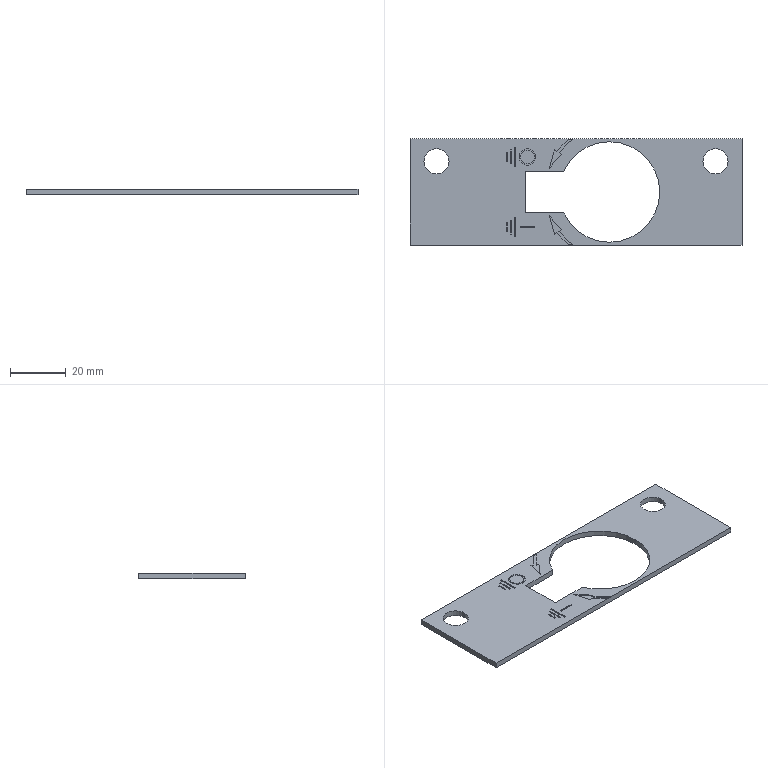Part | STEP file | Earthing switch operating hole label | 1 solid | 73 faces | box 119 x 38 x 2 mm | volume 6366 mm3 | plane 59 | cylinder 14 | commonest cylinder face diameters 9 x4 5 x2 6 x2 36 x2 46.386 x2 48.386 x2